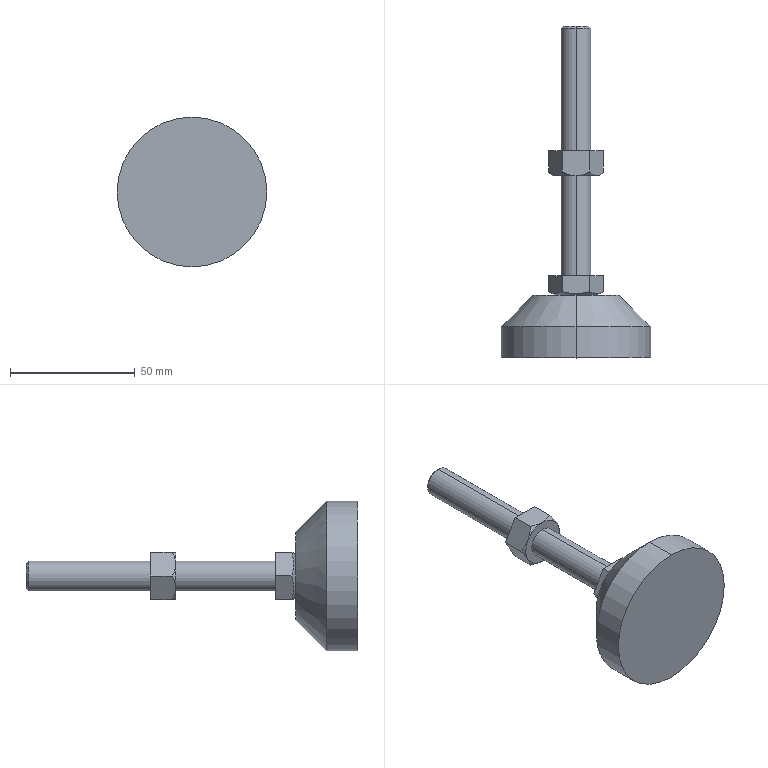Part | STEP file | FBR60-12-100 | 2 solids | 45 faces | box 60 x 133 x 60 mm | volume 73980 mm3 | plane 18 | cone 16 | cylinder 10 | spline 1 | commonest cylinder face diameters 10.106 x2 12 x2 27 x2 35 x2 60 x2